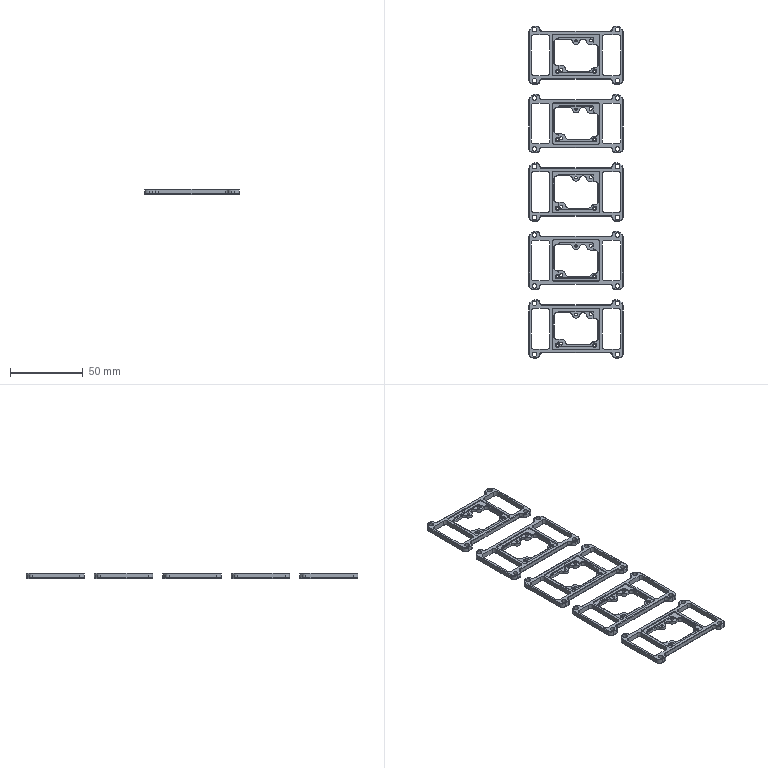NC program | NX | posted with a generic post | part box 65 x 228 x 3.5 mm
Whole program:
N10 G17 G21 G94 G90
(FLOOR_WALL_COPY , TOOL : D80)
N12 T19 M6
N14 G54
N16 G17 G0 G90 X-157. Y0. S6500 M3
N18 G43 Z30. H19
N20 Z4.666
N22 G94 G1 Z1.666 F1500.
N24 X-154.
N26 X154.
N28 X157.
N30 Z4.666
N32 G0 Z30.
N34 X-157.
N36 Z3.833
N38 G1 Z0.833
N40 X-154.
N42 X154.
N44 X157.
N46 Z3.833
N48 G0 Z30.
N50 X-157.
N52 Z3.
N54 G1 Z0.
N56 X-154.
N58 X154.
N60 X157.
N62 Z3.
N64 G0 Z30.
N66 M5
(PLANAR_MILL_COPY_COPY , TOOL : D6A45)
N68 T01 M6
N70 G54
N72 G17 G0 G90 X111.95 Y-28.933 S9500 M3
N74 G43 Z30. H1
N76 Z0.5
N78 G94 G1 Z-1. F1250.
N80 G3 X112.2 Y-28.5 R0.5
N82 X111.5 Y-27.8 R0.7
N84 X112.2 Y-28.5 R-0.7
N86 X111.95 Y-28.067 R0.5
N88 G1 Z0.5
N90 G0 Z30.
N92 X93.134 Y-29.475
N94 Z0.5
N96 G1 Z-1.
N98 G3 X94. Y-29.975 R1.
N100 G1 X106.
N102 G3 X107.1 Y-28.875 R1.1
N104 G1 Y-19.875
N106 G3 X106. Y-18.775 R1.1
N108 G1 X82.
N110 G3 X80.9 Y-19.875 R1.1
N112 G1 Y-28.875
N114 G3 X82. Y-29.975 R1.1
N116 G1 X94.
N118 G3 X94.866 Y-29.475 R1.
N120 G1 Z0.5
N122 G0 Z30.
N124 X83.833 Y-10.225
N126 Z0.5
N128 G1 X83.992 Z0.458
N130 X84.025 Y-10.192 Z0.445
N132 X83.992 Y-9.975 Z0.383
N134 X83.775 Y-10.008 Z0.321
N136 X83.808 Y-10.225 Z0.26
N138 X84.025 Y-10.192 Z0.198
N140 X83.992 Y-9.975 Z0.136
N142 X83.775 Y-10.008 Z0.074
N144 X83.808 Y-10.225 Z0.013
N146 X84.025 Y-10.192 Z-0.049
N148 X83.992 Y-9.975 Z-0.111
N150 X83.775 Y-10.008 Z-0.173
N152 X83.808 Y-10.225 Z-0.234
N154 X84.025 Y-10.192 Z-0.296
N156 X83.992 Y-9.975 Z-0.358
N158 X83.775 Y-10.008 Z-0.42
N160 X83.808 Y-10.225 Z-0.481
N162 X84.025 Y-10.192 Z-0.543
N164 X83.992 Y-9.975 Z-0.605
N166 X83.775 Y-10.008 Z-0.667
N168 X83.808 Y-10.225 Z-0.728
N170 X84.025 Y-10.192 Z-0.79
N172 X83.992 Y-9.975 Z-0.852
N174 X83.775 Y-10.008 Z-0.914
N176 X83.808 Y-10.225 Z-0.975
N178 X83.9 Z-1.
N180 G3 X84.025 Y-10.1 R0.125
N182 X83.9 Y-10.225 R-0.125
N184 G1 Z0.5
N186 G0 Z30.
N188 X95.084 Y-13.6
N190 Z0.5
N192 G1 Z-1.
N194 G3 X95.95 Y-14.1 R1.
N196 G1 X103.
N198 G3 X104.1 Y-13. R1.1
N200 G1 Y-4.419
N202 G3 X103.208 Y-3.339 R1.1
N204 G2 X103.208 Y3.339 R3.4
N206 G3 X104.1 Y4.419 R1.1
N208 G1 Y5.223
N210 G3 X103.242 Y6.296 R1.1
N212 G2 X100.2 Y10.1 R3.9
N214 G1 Y13.
N216 G3 X99.1 Y14.1 R1.1
N218 G1 X87.34
N220 G3 X86.242 Y12.927 R1.1
N222 G2 X84.474 Y9.713 R3.4
N224 G3 X83.9 Y8.747 R1.1
N226 G1 Y-5.223
N228 G3 X84.758 Y-6.296 R1.1
N230 G2 X87.8 Y-10.1 R3.9
N232 G1 Y-13.
N234 G3 X88.9 Y-14.1 R1.1
N236 G1 X95.95
N238 G3 X96.816 Y-13.6 R1.
N240 G1 Z0.5
N242 G0 Z30.
N244 X111.9 Y0.866
N246 Z0.5
N248 G1 Z-1.
N250 G3 X111.4 Y0. R1.
N252 G1 Y-23.
N254 G3 X112.363 Y-24.091 R1.1
N256 G2 X114.9 Y-26.969 R2.9
N258 G1 Y-28.257
N260 G2 X113.758 Y-31.015 R3.9
N262 G1 X112.515 Y-32.258
N264 G2 X109.757 Y-33.4 R3.9
N266 G1 X77.
N268 G2 X73.1 Y-29.5 R3.9
N270 G1 Y-26.969
N272 G2 X75.638 Y-24.091 R2.9
N274 G3 X76.6 Y-23. R1.1
N276 G1 Y23.
N278 G3 X75.638 Y24.091 R1.1
N280 G2 X73.1 Y26.969 R2.9
N282 G1 Y29.5
N284 G2 X77. Y33.4 R3.9
N286 G1 X109.757
N288 G2 X112.515 Y32.258 R3.9
N290 G1 X113.758 Y31.015
N292 G2 X114.9 Y28.257 R3.9
N294 G1 Y26.969
N296 G2 X112.363 Y24.091 R2.9
N298 G3 X111.4 Y23. R1.1
N300 G1 Y0.
N302 G3 X111.9 Y-0.866 R1.
N304 G1 Z0.5
N306 G0 Z30.
N308 X104.225 Y10.033
N310 Z0.5
N312 G1 Y10.192 Z0.458
N314 X104.192 Y10.225 Z0.445
N316 X103.975 Y10.192 Z0.383
N318 X104.008 Y9.975 Z0.321
N320 X104.225 Y10.008 Z0.26
N322 X104.192 Y10.225 Z0.198
N324 X103.975 Y10.192 Z0.136
N326 X104.008 Y9.975 Z0.074
N328 X104.225 Y10.008 Z0.013
N330 X104.192 Y10.225 Z-0.049
N332 X103.975 Y10.192 Z-0.111
N334 X104.008 Y9.975 Z-0.173
N336 X104.225 Y10.008 Z-0.234
N338 X104.192 Y10.225 Z-0.296
N340 X103.975 Y10.192 Z-0.358
N342 X104.008 Y9.975 Z-0.42
N344 X104.225 Y10.008 Z-0.481
N346 X104.192 Y10.225 Z-0.543
N348 X103.975 Y10.192 Z-0.605
N350 X104.008 Y9.975 Z-0.667
N352 X104.225 Y10.008 Z-0.728
N354 X104.192 Y10.225 Z-0.79
N356 X103.975 Y10.192 Z-0.852
N358 X104.008 Y9.975 Z-0.914
N360 X104.225 Y10.008 Z-0.975
N362 Y10.1 Z-1.
N364 G3 X104.1 Y10.225 R0.125
N366 X104.225 Y10.1 R-0.125
N368 G1 Z0.5
N370 G0 Z30.
N372 X111.95 Y28.067
N374 Z0.5
N376 G1 Z-1.
N378 G3 X112.2 Y28.5 R0.5
N380 X111.5 Y29.2 R0.7
N382 X112.2 Y28.5 R-0.7
N384 X111.95 Y28.933 R0.5
N386 G1 Z0.5
N388 G0 Z30.
N390 X94.866 Y29.475
N392 Z0.5
N394 G1 Z-1.
N396 G3 X94. Y29.975 R1.
N398 G1 X82.
N400 G3 X80.9 Y28.875 R1.1
N402 G1 Y19.875
N404 G3 X82. Y18.775 R1.1
N406 G1 X106.
N408 G3 X107.1 Y19.875 R1.1
N410 G1 Y28.875
N412 G3 X106. Y29.975 R1.1
N414 G1 X94.
N416 G3 X93.134 Y29.475 R1.
N418 G1 Z0.5
N420 G0 Z30.
N422 X76.933 Y28.95
N424 Z0.5
N426 G1 Z-1.
N428 G3 X76.5 Y29.2 R0.5
N430 X75.8 Y28.5 R0.7
N432 X76.5 Y29.2 R-0.7
N434 X76.067 Y28.95 R0.5
N436 G1 Z0.5
N438 G0 Z30.
N440 X64.933
N442 Z0.5
N444 G1 Z-1.
N446 G3 X64.5 Y29.2 R0.5
N448 X63.8 Y28.5 R0.7
N450 X64.5 Y29.2 R-0.7
N452 X64.067 Y28.95 R0.5
N454 G1 Z0.5
N456 G0 Z30.
N458 X57.167 Y10.225
N460 Z0.5
N462 G1 X57.008 Z0.458
N464 X56.975 Y10.192 Z0.445
N466 X57.008 Y9.975 Z0.383
N468 X57.225 Y10.008 Z0.321
N470 X57.192 Y10.225 Z0.26
N472 X56.975 Y10.192 Z0.198
N474 X57.008 Y9.975 Z0.136
N476 X57.225 Y10.008 Z0.074
N478 X57.192 Y10.225 Z0.013
N480 X56.975 Y10.192 Z-0.049
N482 X57.008 Y9.975 Z-0.111
N484 X57.225 Y10.008 Z-0.173
N486 X57.192 Y10.225 Z-0.234
N488 X56.975 Y10.192 Z-0.296
N490 X57.008 Y9.975 Z-0.358
N492 X57.225 Y10.008 Z-0.42
N494 X57.192 Y10.225 Z-0.481
N496 X56.975 Y10.192 Z-0.543
N498 X57.008 Y9.975 Z-0.605
N500 X57.225 Y10.008 Z-0.667
N502 X57.192 Y10.225 Z-0.728
N504 X56.975 Y10.192 Z-0.79
N506 X57.008 Y9.975 Z-0.852
N508 X57.225 Y10.008 Z-0.914
N510 X57.192 Y10.225 Z-0.975
N512 X57.1 Z-1.
N514 G3 X56.975 Y10.1 R0.125
N516 X57.1 Y10.225 R-0.125
N518 G1 Z0.5
N520 G0 Z30.
N522 X47.866 Y29.475
N524 Z0.5
N526 G1 Z-1.
N528 G3 X47. Y29.975 R1.
N530 G1 X35.
N532 G3 X33.9 Y28.875 R1.1
N534 G1 Y19.875
N536 G3 X35. Y18.775 R1.1
N538 G1 X59.
N540 G3 X60.1 Y19.875 R1.1
N542 G1 Y28.875
N544 G3 X59. Y29.975 R1.1
N546 G1 X47.
N548 G3 X46.134 Y29.475 R1.
N550 G1 Z0.5
N552 G0 Z30.
N554 X29.933 Y28.95
N556 Z0.5
N558 G1 Z-1.
N560 G3 X29.5 Y29.2 R0.5
N562 X28.8 Y28.5 R0.7
N564 X29.5 Y29.2 R-0.7
N566 X29.067 Y28.95 R0.5
N568 G1 Z0.5
N570 G0 Z30.
N572 X17.933
N574 Z0.5
N576 G1 Z-1.
N578 G3 X17.5 Y29.2 R0.5
N580 X16.8 Y28.5 R0.7
N582 X17.5 Y29.2 R-0.7
N584 X17.067 Y28.95 R0.5
N586 G1 Z0.5
N588 G0 Z30.
N590 X10.167 Y10.225
N592 Z0.5
N594 G1 X10.008 Z0.458
N596 X9.975 Y10.192 Z0.445
N598 X10.008 Y9.975 Z0.383
N600 X10.225 Y10.008 Z0.321
N602 X10.192 Y10.225 Z0.26
N604 X9.975 Y10.192 Z0.198
N606 X10.008 Y9.975 Z0.136
N608 X10.225 Y10.008 Z0.074
N610 X10.192 Y10.225 Z0.013
N612 X9.975 Y10.192 Z-0.049
N614 X10.008 Y9.975 Z-0.111
N616 X10.225 Y10.008 Z-0.173
N618 X10.192 Y10.225 Z-0.234
N620 X9.975 Y10.192 Z-0.296
N622 X10.008 Y9.975 Z-0.358
N624 X10.225 Y10.008 Z-0.42
N626 X10.192 Y10.225 Z-0.481
N628 X9.975 Y10.192 Z-0.543
N630 X10.008 Y9.975 Z-0.605
N632 X10.225 Y10.008 Z-0.667
N634 X10.192 Y10.225 Z-0.728
N636 X9.975 Y10.192 Z-0.79
N638 X10.008 Y9.975 Z-0.852
N640 X10.225 Y10.008 Z-0.914
N642 X10.192 Y10.225 Z-0.975
N644 X10.1 Z-1.
N646 G3 X9.975 Y10.1 R0.125
N648 X10.1 Y10.225 R-0.125
N650 G1 Z0.5
N652 G0 Z30.
N654 X0.866 Y29.475
N656 Z0.5
N658 G1 Z-1.
N660 G3 X0. Y29.975 R1.
N662 G1 X-12.
N664 G3 X-13.1 Y28.875 R1.1
N666 G1 Y19.875
N668 G3 X-12. Y18.775 R1.1
N670 G1 X12.
N672 G3 X13.1 Y19.875 R1.1
N674 G1 Y28.875
N676 G3 X12. Y29.975 R1.1
N678 G1 X0.
N680 G3 X-0.866 Y29.475 R1.
N682 G1 Z0.5
N684 G0 Z30.
N686 X-17.067 Y28.95
N688 Z0.5
N690 G1 Z-1.
N692 G3 X-17.5 Y29.2 R0.5
N694 X-18.2 Y28.5 R0.7
N696 X-17.5 Y29.2 R-0.7
N698 X-17.933 Y28.95 R0.5
N700 G1 Z0.5
N702 G0 Z30.
N704 X-29.067
N706 Z0.5
N708 G1 Z-1.
N710 G3 X-29.5 Y29.2 R0.5
N712 X-30.2 Y28.5 R0.7
N714 X-29.5 Y29.2 R-0.7
N716 X-29.933 Y28.95 R0.5
N718 G1 Z0.5
N720 G0 Z30.
N722 X-36.833 Y10.225
N724 Z0.5
N726 G1 X-36.992 Z0.458
N728 X-37.025 Y10.192 Z0.445
N730 X-36.992 Y9.975 Z0.383
N732 X-36.775 Y10.008 Z0.321
N734 X-36.808 Y10.225 Z0.26
N736 X-37.025 Y10.192 Z0.198
N738 X-36.992 Y9.975 Z0.136
N740 X-36.775 Y10.008 Z0.074
N742 X-36.808 Y10.225 Z0.013
N744 X-37.025 Y10.192 Z-0.049
N746 X-36.992 Y9.975 Z-0.111
N748 X-36.775 Y10.008 Z-0.173
N750 X-36.808 Y10.225 Z-0.234
N752 X-37.025 Y10.192 Z-0.296
N754 X-36.992 Y9.975 Z-0.358
N756 X-36.775 Y10.008 Z-0.42
N758 X-36.808 Y10.225 Z-0.481
N760 X-37.025 Y10.192 Z-0.543
N762 X-36.992 Y9.975 Z-0.605
N764 X-36.775 Y10.008 Z-0.667
N766 X-36.808 Y10.225 Z-0.728
N768 X-37.025 Y10.192 Z-0.79
N770 X-36.992 Y9.975 Z-0.852
N772 X-36.775 Y10.008 Z-0.914
N774 X-36.808 Y10.225 Z-0.975
N776 X-36.9 Z-1.
N778 G3 X-37.025 Y10.1 R0.125
N780 X-36.9 Y10.225 R-0.125
N782 G1 Z0.5
N784 G0 Z30.
N786 X-46.134 Y29.475
N788 Z0.5
N790 G1 Z-1.
N792 G3 X-47. Y29.975 R1.
N794 G1 X-59.
N796 G3 X-60.1 Y28.875 R1.1
N798 G1 Y19.875
N800 G3 X-59. Y18.775 R1.1
N802 G1 X-35.
N804 G3 X-33.9 Y19.875 R1.1
N806 G1 Y28.875
N808 G3 X-35. Y29.975 R1.1
N810 G1 X-47.
N812 G3 X-47.866 Y29.475 R1.
N814 G1 Z0.5
N816 G0 Z30.
N818 X-64.067 Y28.95
N820 Z0.5
N822 G1 Z-1.
N824 G3 X-64.5 Y29.2 R0.5
N826 X-65.2 Y28.5 R0.7
N828 X-64.5 Y29.2 R-0.7
N830 X-64.933 Y28.95 R0.5
N832 G1 Z0.5
N834 G0 Z30.
N836 X-76.067
N838 Z0.5
N840 G1 Z-1.
N842 G3 X-76.5 Y29.2 R0.5
N844 X-77.2 Y28.5 R0.7
N846 X-76.5 Y29.2 R-0.7
N848 X-76.933 Y28.95 R0.5
N850 G1 Z0.5
N852 G0 Z30.
N854 X-93.134 Y29.475
N856 Z0.5
N858 G1 Z-1.
N860 G3 X-94. Y29.975 R1.
N862 G1 X-106.
N864 G3 X-107.1 Y28.875 R1.1
N866 G1 Y19.875
N868 G3 X-106. Y18.775 R1.1
N870 G1 X-82.
N872 G3 X-80.9 Y19.875 R1.1
N874 G1 Y28.875
N876 G3 X-82. Y29.975 R1.1
N878 G1 X-94.
N880 G3 X-94.866 Y29.475 R1.
N882 G1 Z0.5
N884 G0 Z30.
N886 X-111.95 Y28.933
N888 Z0.5
N890 G1 Z-1.
N892 G3 X-112.2 Y28.5 R0.5
N894 X-111.5 Y27.8 R0.7
N896 X-112.2 Y28.5 R-0.7
N898 X-111.95 Y28.067 R0.5
N900 G1 Z0.5
N902 G0 Z30.
N904 X-83.833 Y10.225
N906 Z0.5
N908 G1 X-83.992 Z0.458
N910 X-84.025 Y10.192 Z0.445
N912 X-83.992 Y9.975 Z0.383
N914 X-83.775 Y10.008 Z0.321
N916 X-83.808 Y10.225 Z0.26
N918 X-84.025 Y10.192 Z0.198
N920 X-83.992 Y9.975 Z0.136
N922 X-83.775 Y10.008 Z0.074
N924 X-83.808 Y10.225 Z0.013
N926 X-84.025 Y10.192 Z-0.049
N928 X-83.992 Y9.975 Z-0.111
N930 X-83.775 Y10.008 Z-0.173
N932 X-83.808 Y10.225 Z-0.234
N934 X-84.025 Y10.192 Z-0.296
N936 X-83.992 Y9.975 Z-0.358
N938 X-83.775 Y10.008 Z-0.42
N940 X-83.808 Y10.225 Z-0.481
N942 X-84.025 Y10.192 Z-0.543
N944 X-83.992 Y9.975 Z-0.605
N946 X-83.775 Y10.008 Z-0.667
N948 X-83.808 Y10.225 Z-0.728
N950 X-84.025 Y10.192 Z-0.79
N952 X-83.992 Y9.975 Z-0.852
N954 X-83.775 Y10.008 Z-0.914
N956 X-83.808 Y10.225 Z-0.975
N958 X-83.9 Z-1.
N960 G3 X-84.025 Y10.1 R0.125
N962 X-83.9 Y10.225 R-0.125
N964 G1 Z0.5
N966 G0 Z30.
N968 X-111.9 Y-0.866
N970 Z0.5
N972 G1 Z-1.
N974 G3 X-111.4 Y0. R1.
N976 G1 Y23.
N978 G3 X-112.363 Y24.091 R1.1
N980 G2 X-114.9 Y26.969 R2.9
N982 G1 Y29.5
N984 G2 X-111. Y33.4 R3.9
N986 G1 X-78.243
N988 G2 X-75.485 Y32.258 R3.9
N990 G1 X-74.242 Y31.015
N992 G2 X-73.1 Y28.257 R3.9
N994 G1 Y26.969
N996 G2 X-75.638 Y24.091 R2.9
N998 G3 X-76.6 Y23. R1.1
N1000 G1 Y-23.
N1002 G3 X-75.638 Y-24.091 R1.1
N1004 G2 X-73.1 Y-26.969 R2.9
N1006 G1 Y-28.257
N1008 G2 X-74.242 Y-31.015 R3.9
N1010 G1 X-75.485 Y-32.258
N1012 G2 X-78.243 Y-33.4 R3.9
N1014 G1 X-111.
N1016 G2 X-114.9 Y-29.5 R3.9
N1018 G1 Y-26.969
N1020 G2 X-112.363 Y-24.091 R2.9
N1022 G3 X-111.4 Y-23. R1.1
N1024 G1 Y0.
N1026 G3 X-111.9 Y0.866 R1.
N1028 G1 Z0.5
N1030 G0 Z30.
N1032 X-103.6 Y2.628
N1034 Z0.5
N1036 G1 Z-1.
N1038 G3 X-104.1 Y1.762 R1.
N1040 G1 Y-5.223
N1042 G3 X-103.242 Y-6.296 R1.1
N1044 G2 X-100.2 Y-10.1 R3.9
N1046 G1 Y-13.
N1048 G3 X-99.1 Y-14.1 R1.1
N1050 G1 X-85.
N1052 G3 X-83.9 Y-13. R1.1
N1054 G1 Y-4.419
N1056 G3 X-84.792 Y-3.339 R1.1
N1058 G2 X-84.792 Y3.339 R3.4
N1060 G3 X-83.9 Y4.419 R1.1
N1062 G1 Y5.223
N1064 G3 X-84.758 Y6.296 R1.1
N1066 G2 X-87.8 Y10.1 R3.9
N1068 G1 Y13.
N1070 G3 X-88.9 Y14.1 R1.1
N1072 G1 X-100.66
N1074 G3 X-101.758 Y12.927 R1.1
N1076 G2 X-103.526 Y9.713 R3.4
N1078 G3 X-104.1 Y8.747 R1.1
N1080 G1 Y1.762
N1082 G3 X-103.6 Y0.896 R1.
N1084 G1 Z0.5
N1086 G0 Z30.
N1088 X-104.225 Y-10.033
N1090 Z0.5
N1092 G1 Y-10.192 Z0.458
N1094 X-104.192 Y-10.225 Z0.445
N1096 X-103.975 Y-10.192 Z0.383
N1098 X-104.008 Y-9.975 Z0.321
N1100 X-104.225 Y-10.008 Z0.26
N1102 X-104.192 Y-10.225 Z0.198
N1104 X-103.975 Y-10.192 Z0.136
N1106 X-104.008 Y-9.975 Z0.074
N1108 X-104.225 Y-10.008 Z0.013
N1110 X-104.192 Y-10.225 Z-0.049
N1112 X-103.975 Y-10.192 Z-0.111
N1114 X-104.008 Y-9.975 Z-0.173
N1116 X-104.225 Y-10.008 Z-0.234
N1118 X-104.192 Y-10.225 Z-0.296
N1120 X-103.975 Y-10.192 Z-0.358
N1122 X-104.008 Y-9.975 Z-0.42
N1124 X-104.225 Y-10.008 Z-0.481
N1126 X-104.192 Y-10.225 Z-0.543
N1128 X-103.975 Y-10.192 Z-0.605
N1130 X-104.008 Y-9.975 Z-0.667
N1132 X-104.225 Y-10.008 Z-0.728
N1134 X-104.192 Y-10.225 Z-0.79
N1136 X-103.975 Y-10.192 Z-0.852
N1138 X-104.008 Y-9.975 Z-0.914
N1140 X-104.225 Y-10.008 Z-0.975
N1142 Y-10.1 Z-1.
N1144 G3 X-104.1 Y-10.225 R0.125
N1146 X-104.225 Y-10.1 R-0.125
N1148 G1 Z0.5
N1150 G0 Z30.
N1152 X-111.95 Y-28.067
N1154 Z0.5
N1156 G1 Z-1.
N1158 G3 X-112.2 Y-28.5 R0.5
N1160 X-111.5 Y-29.2 R0.7
N1162 X-112.2 Y-28.5 R-0.7
N1164 X-111.95 Y-28.933 R0.5
N1166 G1 Z0.5
N1168 G0 Z30.
N1170 X-94.866 Y-29.475
N1172 Z0.5
N1174 G1 Z-1.
N1176 G3 X-94. Y-29.975 R1.
N1178 G1 X-82.
N1180 G3 X-80.9 Y-28.875 R1.1
N1182 G1 Y-19.875
N1184 G3 X-82. Y-18.775 R1.1
N1186 G1 X-106.
N1188 G3 X-107.1 Y-19.875 R1.1
N1190 G1 Y-28.875
N1192 G3 X-106. Y-29.975 R1.1
N1194 G1 X-94.
N1196 G3 X-93.134 Y-29.475 R1.
N1198 G1 Z0.5
N1200 G0 Z30.
N1202 X-76.933 Y-28.95
N1204 Z0.5
N1206 G1 Z-1.
N1208 G3 X-76.5 Y-29.2 R0.5
N1210 X-75.8 Y-28.5 R0.7
N1212 X-76.5 Y-29.2 R-0.7
N1214 X-76.067 Y-28.95 R0.5
N1216 G1 Z0.5
N1218 G0 Z30.
N1220 X-64.933
N1222 Z0.5
N1224 G1 Z-1.
N1226 G3 X-64.5 Y-29.2 R0.5
N1228 X-63.8 Y-28.5 R0.7
N1230 X-64.5 Y-29.2 R-0.7
N1232 X-64.067 Y-28.95 R0.5
N1234 G1 Z0.5
N1236 G0 Z30.
N1238 X-57.167 Y-10.225
N1240 Z0.5
N1242 G1 X-57.008 Z0.458
N1244 X-56.975 Y-10.192 Z0.445
N1246 X-57.008 Y-9.975 Z0.383
N1248 X-57.225 Y-10.008 Z0.321
N1250 X-57.192 Y-10.225 Z0.26
N1252 X-56.975 Y-10.192 Z0.198
N1254 X-57.008 Y-9.975 Z0.136
N1256 X-57.225 Y-10.008 Z0.074
N1258 X-57.192 Y-10.225 Z0.013
N1260 X-56.975 Y-10.192 Z-0.049
N1262 X-57.008 Y-9.975 Z-0.111
N1264 X-57.225 Y-10.008 Z-0.173
N1266 X-57.192 Y-10.225 Z-0.234
N1268 X-56.975 Y-10.192 Z-0.296
N1270 X-57.008 Y-9.975 Z-0.358
N1272 X-57.225 Y-10.008 Z-0.42
N1274 X-57.192 Y-10.225 Z-0.481
N1276 X-56.975 Y-10.192 Z-0.543
N1278 X-57.008 Y-9.975 Z-0.605
N1280 X-57.225 Y-10.008 Z-0.667
N1282 X-57.192 Y-10.225 Z-0.728
N1284 X-56.975 Y-10.192 Z-0.79
N1286 X-57.008 Y-9.975 Z-0.852
N1288 X-57.225 Y-10.008 Z-0.914
N1290 X-57.192 Y-10.225 Z-0.975
N1292 X-57.1 Z-1.
N1294 G3 X-56.975 Y-10.1 R0.125
N1296 X-57.1 Y-10.225 R-0.125
N1298 G1 Z0.5
N1300 G0 Z30.
N1302 X-64.9 Y-0.866
N1304 Z0.5
N1306 G1 Z-1.
N1308 G3 X-64.4 Y0. R1.
N1310 G1 Y23.
N1312 G3 X-65.363 Y24.091 R1.1
N1314 G2 X-67.9 Y26.969 R2.9
N1316 G1 Y29.5
N1318 G2 X-64. Y33.4 R3.9
N1320 G1 X-31.243
N1322 G2 X-28.485 Y32.258 R3.9
N1324 G1 X-27.242 Y31.015
N1326 G2 X-26.1 Y28.257 R3.9
N1328 G1 Y26.969
N1330 G2 X-28.638 Y24.091 R2.9
N1332 G3 X-29.6 Y23. R1.1
N1334 G1 Y-23.
N1336 G3 X-28.638 Y-24.091 R1.1
N1338 G2 X-26.1 Y-26.969 R2.9
N1340 G1 Y-28.257
N1342 G2 X-27.242 Y-31.015 R3.9
N1344 G1 X-28.485 Y-32.258
N1346 G2 X-31.243 Y-33.4 R3.9
N1348 G1 X-64.
N1350 G2 X-67.9 Y-29.5 R3.9
N1352 G1 Y-26.969
N1354 G2 X-65.363 Y-24.091 R2.9
N1356 G3 X-64.4 Y-23. R1.1
N1358 G1 Y0.
N1360 G3 X-64.9 Y0.866 R1.
N1362 G1 Z0.5
N1364 G0 Z30.
N1366 X-45.916 Y-13.6
N1368 Z0.5
N1370 G1 Z-1.
N1372 G3 X-45.05 Y-14.1 R1.
N1374 G1 X-38.
N1376 G3 X-36.9 Y-13. R1.1
N1378 G1 Y-4.419
N1380 G3 X-37.792 Y-3.339 R1.1
N1382 G2 X-37.792 Y3.339 R3.4
N1384 G3 X-36.9 Y4.419 R1.1
N1386 G1 Y5.223
N1388 G3 X-37.758 Y6.296 R1.1
N1390 G2 X-40.8 Y10.1 R3.9
N1392 G1 Y13.
N1394 G3 X-41.9 Y14.1 R1.1
N1396 G1 X-53.66
N1398 G3 X-54.758 Y12.927 R1.1
N1400 G2 X-56.526 Y9.713 R3.4
N1402 G3 X-57.1 Y8.747 R1.1
N1404 G1 Y-5.223
N1406 G3 X-56.242 Y-6.296 R1.1
N1408 G2 X-53.2 Y-10.1 R3.9
N1410 G1 Y-13.
N1412 G3 X-52.1 Y-14.1 R1.1
N1414 G1 X-45.05
N1416 G3 X-44.184 Y-13.6 R1.
N1418 G1 Z0.5
N1420 G0 Z30.
N1422 X-47.866 Y-29.475
N1424 Z0.5
N1426 G1 Z-1.
N1428 G3 X-47. Y-29.975 R1.
N1430 G1 X-35.
N1432 G3 X-33.9 Y-28.875 R1.1
N1434 G1 Y-19.875
N1436 G3 X-35. Y-18.775 R1.1
N1438 G1 X-59.
N1440 G3 X-60.1 Y-19.875 R1.1
N1442 G1 Y-28.875
N1444 G3 X-59. Y-29.975 R1.1
N1446 G1 X-47.
N1448 G3 X-46.134 Y-29.475 R1.
N1450 G1 Z0.5
N1452 G0 Z30.
N1454 X-29.933 Y-28.95
N1456 Z0.5
N1458 G1 Z-1.
N1460 G3 X-29.5 Y-29.2 R0.5
N1462 X-28.8 Y-28.5 R0.7
N1464 X-29.5 Y-29.2 R-0.7
N1466 X-29.067 Y-28.95 R0.5
N1468 G1 Z0.5
N1470 G0 Z30.
N1472 X-17.933
N1474 Z0.5
N1476 G1 Z-1.
N1478 G3 X-17.5 Y-29.2 R0.5
N1480 X-16.8 Y-28.5 R0.7
N1482 X-17.5 Y-29.2 R-0.7
N1484 X-17.067 Y-28.95 R0.5
N1486 G1 Z0.5
N1488 G0 Z30.
N1490 X-10.167 Y-10.225
N1492 Z0.5
N1494 G1 X-10.008 Z0.458
N1496 X-9.975 Y-10.192 Z0.445
N1498 X-10.008 Y-9.975 Z0.383
N1500 X-10.225 Y-10.008 Z0.321
N1502 X-10.192 Y-10.225 Z0.26
N1504 X-9.975 Y-10.192 Z0.198
N1506 X-10.008 Y-9.975 Z0.136
N1508 X-10.225 Y-10.008 Z0.074
N1510 X-10.192 Y-10.225 Z0.013
N1512 X-9.975 Y-10.192 Z-0.049
N1514 X-10.008 Y-9.975 Z-0.111
N1516 X-10.225 Y-10.008 Z-0.173
N1518 X-10.192 Y-10.225 Z-0.234
N1520 X-9.975 Y-10.192 Z-0.296
N1522 X-10.008 Y-9.975 Z-0.358
N1524 X-10.225 Y-10.008 Z-0.42
N1526 X-10.192 Y-10.225 Z-0.481
N1528 X-9.975 Y-10.192 Z-0.543
N1530 X-10.008 Y-9.975 Z-0.605
N1532 X-10.225 Y-10.008 Z-0.667
N1534 X-10.192 Y-10.225 Z-0.728
N1536 X-9.975 Y-10.192 Z-0.79
N1538 X-10.008 Y-9.975 Z-0.852
N1540 X-10.225 Y-10.008 Z-0.914
N1542 X-10.192 Y-10.225 Z-0.975
N1544 X-10.1 Z-1.
N1546 G3 X-9.975 Y-10.1 R0.125
N1548 X-10.1 Y-10.225 R-0.125
N1550 G1 Z0.5
N1552 G0 Z30.
N1554 X-17.9 Y-0.866
N1556 Z0.5
N1558 G1 Z-1.
N1560 G3 X-17.4 Y0. R1.
N1562 G1 Y23.
N1564 G3 X-18.363 Y24.091 R1.1
N1566 G2 X-20.9 Y26.969 R2.9
N1568 G1 Y29.5
N1570 G2 X-17. Y33.4 R3.9
N1572 G1 X15.757
N1574 G2 X18.515 Y32.258 R3.9
N1576 G1 X19.758 Y31.015
N1578 G2 X20.9 Y28.257 R3.9
N1580 G1 Y26.969
N1582 G2 X18.363 Y24.091 R2.9
N1584 G3 X17.4 Y23. R1.1
N1586 G1 Y-23.
N1588 G3 X18.363 Y-24.091 R1.1
N1590 G2 X20.9 Y-26.969 R2.9
N1592 G1 Y-28.257
N1594 G2 X19.758 Y-31.015 R3.9
N1596 G1 X18.515 Y-32.258
N1598 G2 X15.757 Y-33.4 R3.9
N1600 G1 X-17.
N1602 G2 X-20.9 Y-29.5 R3.9
N1604 G1 Y-26.969
N1606 G2 X-18.363 Y-24.091 R2.9
N1608 G3 X-17.4 Y-23. R1.1
N1610 G1 Y0.
N1612 G3 X-17.9 Y0.866 R1.
N1614 G1 Z0.5
N1616 G0 Z30.
N1618 X1.084 Y-13.6
N1620 Z0.5
N1622 G1 Z-1.
N1624 G3 X1.95 Y-14.1 R1.
N1626 G1 X9.
N1628 G3 X10.1 Y-13. R1.1
N1630 G1 Y-4.419
N1632 G3 X9.208 Y-3.339 R1.1
N1634 G2 X9.208 Y3.339 R3.4
N1636 G3 X10.1 Y4.419 R1.1
N1638 G1 Y5.223
N1640 G3 X9.242 Y6.296 R1.1
N1642 G2 X6.2 Y10.1 R3.9
N1644 G1 Y13.
N1646 G3 X5.1 Y14.1 R1.1
N1648 G1 X-6.66
N1650 G3 X-7.758 Y12.927 R1.1
N1652 G2 X-9.526 Y9.713 R3.4
N1654 G3 X-10.1 Y8.747 R1.1
N1656 G1 Y-5.223
N1658 G3 X-9.242 Y-6.296 R1.1
N1660 G2 X-6.2 Y-10.1 R3.9
N1662 G1 Y-13.
N1664 G3 X-5.1 Y-14.1 R1.1
N1666 G1 X1.95
N1668 G3 X2.816 Y-13.6 R1.
N1670 G1 Z0.5
N1672 G0 Z30.
N1674 X-0.866 Y-29.475
N1676 Z0.5
N1678 G1 Z-1.
N1680 G3 X0. Y-29.975 R1.
N1682 G1 X12.
N1684 G3 X13.1 Y-28.875 R1.1
N1686 G1 Y-19.875
N1688 G3 X12. Y-18.775 R1.1
N1690 G1 X-12.
N1692 G3 X-13.1 Y-19.875 R1.1
N1694 G1 Y-28.875
N1696 G3 X-12. Y-29.975 R1.1
N1698 G1 X0.
N1700 G3 X0.866 Y-29.475 R1.
N1702 G1 Z0.5
N1704 G0 Z30.
N1706 X17.067 Y-28.95
N1708 Z0.5
N1710 G1 Z-1.
N1712 G3 X17.5 Y-29.2 R0.5
N1714 X18.2 Y-28.5 R0.7
N1716 X17.5 Y-29.2 R-0.7
N1718 X17.933 Y-28.95 R0.5
N1720 G1 Z0.5
N1722 G0 Z30.
N1724 X29.067
N1726 Z0.5
N1728 G1 Z-1.
N1730 G3 X29.5 Y-29.2 R0.5
N1732 X30.2 Y-28.5 R0.7
N1734 X29.5 Y-29.2 R-0.7
N1736 X29.933 Y-28.95 R0.5
N1738 G1 Z0.5
N1740 G0 Z30.
N1742 X36.833 Y-10.225
N1744 Z0.5
N1746 G1 X36.992 Z0.458
N1748 X37.025 Y-10.192 Z0.445
N1750 X36.992 Y-9.975 Z0.383
N1752 X36.775 Y-10.008 Z0.321
N1754 X36.808 Y-10.225 Z0.26
N1756 X37.025 Y-10.192 Z0.198
N1758 X36.992 Y-9.975 Z0.136
N1760 X36.775 Y-10.008 Z0.074
N1762 X36.808 Y-10.225 Z0.013
N1764 X37.025 Y-10.192 Z-0.049
N1766 X36.992 Y-9.975 Z-0.111
N1768 X36.775 Y-10.008 Z-0.173
N1770 X36.808 Y-10.225 Z-0.234
N1772 X37.025 Y-10.192 Z-0.296
N1774 X36.992 Y-9.975 Z-0.358
N1776 X36.775 Y-10.008 Z-0.42
N1778 X36.808 Y-10.225 Z-0.481
N1780 X37.025 Y-10.192 Z-0.543
N1782 X36.992 Y-9.975 Z-0.605
N1784 X36.775 Y-10.008 Z-0.667
N1786 X36.808 Y-10.225 Z-0.728
N1788 X37.025 Y-10.192 Z-0.79
N1790 X36.992 Y-9.975 Z-0.852
N1792 X36.775 Y-10.008 Z-0.914
N1794 X36.808 Y-10.225 Z-0.975
N1796 X36.9 Z-1.
N1798 G3 X37.025 Y-10.1 R0.125
N1800 X36.9 Y-10.225 R-0.125
N1802 G1 Z0.5
N1804 G0 Z30.
N1806 X29.1 Y-0.866
N1808 Z0.5
N1810 G1 Z-1.
N1812 G3 X29.6 Y0. R1.
N1814 G1 Y23.
N1816 G3 X28.638 Y24.091 R1.1
N1818 G2 X26.1 Y26.969 R2.9
N1820 G1 Y29.5
N1822 G2 X30. Y33.4 R3.9
N1824 G1 X62.757
N1826 G2 X65.515 Y32.258 R3.9
N1828 G1 X66.758 Y31.015
N1830 G2 X67.9 Y28.257 R3.9
N1832 G1 Y26.969
N1834 G2 X65.363 Y24.091 R2.9
N1836 G3 X64.4 Y23. R1.1
N1838 G1 Y-23.
N1840 G3 X65.363 Y-24.091 R1.1
N1842 G2 X67.9 Y-26.969 R2.9
N1844 G1 Y-28.257
N1846 G2 X66.758 Y-31.015 R3.9
N1848 G1 X65.515 Y-32.258
N1850 G2 X62.757 Y-33.4 R3.9
N1852 G1 X30.
N1854 G2 X26.1 Y-29.5 R3.9
N1856 G1 Y-26.969
N1858 G2 X28.638 Y-24.091 R2.9
N1860 G3 X29.6 Y-23. R1.1
N1862 G1 Y0.
N1864 G3 X29.1 Y0.866 R1.
N1866 G1 Z0.5
N1868 G0 Z30.
N1870 X48.084 Y-13.6
N1872 Z0.5
N1874 G1 Z-1.
N1876 G3 X48.95 Y-14.1 R1.
N1878 G1 X56.
N1880 G3 X57.1 Y-13. R1.1
N1882 G1 Y-4.419
N1884 G3 X56.208 Y-3.339 R1.1
N1886 G2 X56.208 Y3.339 R3.4
N1888 G3 X57.1 Y4.419 R1.1
N1890 G1 Y5.223
N1892 G3 X56.242 Y6.296 R1.1
N1894 G2 X53.2 Y10.1 R3.9
N1896 G1 Y13.
N1898 G3 X52.1 Y14.1 R1.1
N1900 G1 X40.34
N1902 G3 X39.242 Y12.927 R1.1
N1904 G2 X37.474 Y9.713 R3.4
N1906 G3 X36.9 Y8.747 R1.1
N1908 G1 Y-5.223
N1910 G3 X37.758 Y-6.296 R1.1
N1912 G2 X40.8 Y-10.1 R3.9
N1914 G1 Y-13.
N1916 G3 X41.9 Y-14.1 R1.1
N1918 G1 X48.95
N1920 G3 X49.816 Y-13.6 R1.
N1922 G1 Z0.5
N1924 G0 Z30.
N1926 X46.134 Y-29.475
N1928 Z0.5
N1930 G1 Z-1.
N1932 G3 X47. Y-29.975 R1.
N1934 G1 X59.
N1936 G3 X60.1 Y-28.875 R1.1
N1938 G1 Y-19.875
N1940 G3 X59. Y-18.775 R1.1
N1942 G1 X35.
N1944 G3 X33.9 Y-19.875 R1.1
N1946 G1 Y-28.875
N1948 G3 X35. Y-29.975 R1.1
N1950 G1 X47.
N1952 G3 X47.866 Y-29.475 R1.
N1954 G1 Z0.5
N1956 G0 Z30.
N1958 X64.067 Y-28.95
N1960 Z0.5
N1962 G1 Z-1.
N1964 G3 X64.5 Y-29.2 R0.5
N1966 X65.2 Y-28.5 R0.7
N1968 X64.5 Y-29.2 R-0.7
N1970 X64.933 Y-28.95 R0.5
N1972 G1 Z0.5
N1974 G0 Z30.
N1976 X76.067
N1978 Z0.5
N1980 G1 Z-1.
N1982 G3 X76.5 Y-29.2 R0.5
N1984 X77.2 Y-28.5 R0.7
N1986 X76.5 Y-29.2 R-0.7
N1988 X76.933 Y-28.95 R0.5
N1990 G1 Z0.5
N1992 G0 Z30.
N1994 M5
N1996 M2